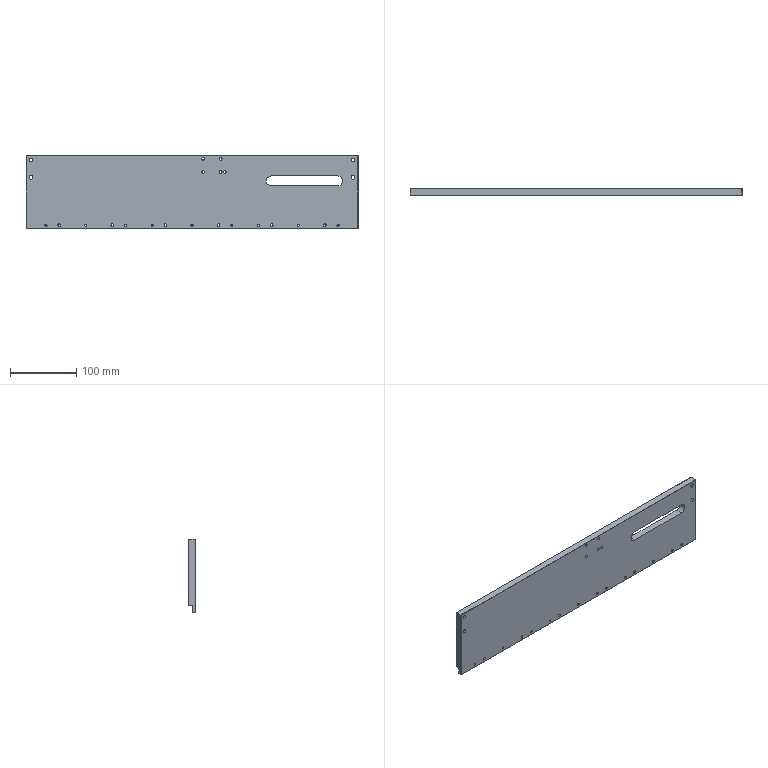Part | NX | 1 solid | 124 faces | box 500 x 10 x 110 mm | volume 502548 mm3 | cylinder 51 | cone 48 | plane 25 | commonest cylinder face diameters 3.3 x18 4 x14 4.2 x8 5.5 x8 15 x3